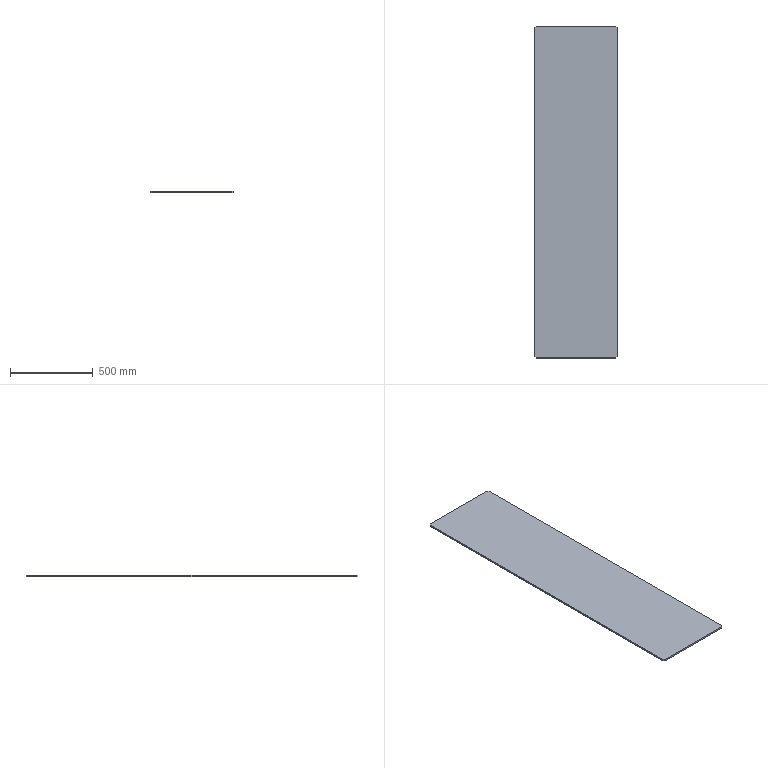Part | SolidWorks | features Chamfer 1, Extrusion 1 | 1 solid | 10 faces | box 500 x 2000 x 10 mm | volume 9998000 mm3 | plane 10
STEP:
#1=CARTESIAN_POINT('',(250.,-990.,5.));
#2=VERTEX_POINT('',#1);
#3=CARTESIAN_POINT('',(250.,990.,5.));
#4=VERTEX_POINT('',#3);
#5=CARTESIAN_POINT('',(250.,-1000.,5.));
#6=DIRECTION('',(0.,1.,0.));
#7=VECTOR('',#6,1000.);
#8=LINE('',#5,#7);
#9=EDGE_CURVE('',#2,#4,#8,.T.);
#10=ORIENTED_EDGE('',*,*,#9,.F.);
#11=CARTESIAN_POINT('',(250.,-990.,-5.));
#12=VERTEX_POINT('',#11);
#13=CARTESIAN_POINT('',(250.,-990.,5.));
#14=DIRECTION('',(0.,0.,-1.));
#15=VECTOR('',#14,1000.);
#16=LINE('',#13,#15);
#17=EDGE_CURVE('',#2,#12,#16,.T.);
#18=ORIENTED_EDGE('',*,*,#17,.T.);
#19=CARTESIAN_POINT('',(250.,990.,-5.));
#20=VERTEX_POINT('',#19);
#21=CARTESIAN_POINT('',(250.,-1000.,-5.));
#22=DIRECTION('',(0.,1.,0.));
#23=VECTOR('',#22,1000.);
#24=LINE('',#21,#23);
#25=EDGE_CURVE('',#12,#20,#24,.T.);
#26=ORIENTED_EDGE('',*,*,#25,.T.);
#27=CARTESIAN_POINT('',(250.,990.,5.));
#28=DIRECTION('',(0.,0.,1.));
#29=VECTOR('',#28,1000.);
#30=LINE('',#27,#29);
#31=EDGE_CURVE('',#20,#4,#30,.T.);
#32=ORIENTED_EDGE('',*,*,#31,.T.);
#33=EDGE_LOOP('',(#10,#18,#26,#32));
#34=FACE_OUTER_BOUND('',#33,.T.);
#35=CARTESIAN_POINT('',(250.,-1000.,5.));
#36=DIRECTION('',(-1.,0.,0.));
#37=DIRECTION('',(0.,0.,1.));
#38=AXIS2_PLACEMENT_3D('',#35,#36,#37);
#39=PLANE('',#38);
#40=ADVANCED_FACE('',(#34),#39,.F.);
#41=CARTESIAN_POINT('',(240.,1000.,-5.));
#42=VERTEX_POINT('',#41);
#43=CARTESIAN_POINT('',(-240.,1000.,-5.));
#44=VERTEX_POINT('',#43);
#45=CARTESIAN_POINT('',(-250.,1000.,-5.));
#46=DIRECTION('',(-1.,0.,0.));
#47=VECTOR('',#46,1000.);
#48=LINE('',#45,#47);
#49=EDGE_CURVE('',#42,#44,#48,.T.);
#50=ORIENTED_EDGE('',*,*,#49,.T.);
#51=CARTESIAN_POINT('',(-240.,1000.,5.));
#52=VERTEX_POINT('',#51);
#53=CARTESIAN_POINT('',(-240.,1000.,5.));
#54=DIRECTION('',(0.,0.,1.));
#55=VECTOR('',#54,1000.);
#56=LINE('',#53,#55);
#57=EDGE_CURVE('',#44,#52,#56,.T.);
#58=ORIENTED_EDGE('',*,*,#57,.T.);
#59=CARTESIAN_POINT('',(240.,1000.,5.));
#60=VERTEX_POINT('',#59);
#61=CARTESIAN_POINT('',(-250.,1000.,5.));
#62=DIRECTION('',(-1.,0.,0.));
#63=VECTOR('',#62,1000.);
#64=LINE('',#61,#63);
#65=EDGE_CURVE('',#60,#52,#64,.T.);
#66=ORIENTED_EDGE('',*,*,#65,.F.);
#67=CARTESIAN_POINT('',(240.,1000.,5.));
#68=DIRECTION('',(0.,0.,-1.));
#69=VECTOR('',#68,1000.);
#70=LINE('',#67,#69);
#71=EDGE_CURVE('',#60,#42,#70,.T.);
#72=ORIENTED_EDGE('',*,*,#71,.T.);
#73=EDGE_LOOP('',(#50,#58,#66,#72));
#74=FACE_OUTER_BOUND('',#73,.T.);
#75=CARTESIAN_POINT('',(-250.,1000.,5.));
#76=DIRECTION('',(0.,-1.,0.));
#77=DIRECTION('',(0.,0.,-1.));
#78=AXIS2_PLACEMENT_3D('',#75,#76,#77);
#79=PLANE('',#78);
#80=ADVANCED_FACE('',(#74),#79,.F.);
#81=CARTESIAN_POINT('',(-250.,990.,5.));
#82=VERTEX_POINT('',#81);
#83=CARTESIAN_POINT('',(-250.,-990.,5.));
#84=VERTEX_POINT('',#83);
#85=CARTESIAN_POINT('',(-250.,-1000.,5.));
#86=DIRECTION('',(0.,-1.,0.));
#87=VECTOR('',#86,1000.);
#88=LINE('',#85,#87);
#89=EDGE_CURVE('',#82,#84,#88,.T.);
#90=ORIENTED_EDGE('',*,*,#89,.F.);
#91=CARTESIAN_POINT('',(-250.,990.,-5.));
#92=VERTEX_POINT('',#91);
#93=CARTESIAN_POINT('',(-250.,990.,5.));
#94=DIRECTION('',(0.,0.,-1.));
#95=VECTOR('',#94,1000.);
#96=LINE('',#93,#95);
#97=EDGE_CURVE('',#82,#92,#96,.T.);
#98=ORIENTED_EDGE('',*,*,#97,.T.);
#99=CARTESIAN_POINT('',(-250.,-990.,-5.));
#100=VERTEX_POINT('',#99);
#101=CARTESIAN_POINT('',(-250.,-1000.,-5.));
#102=DIRECTION('',(0.,-1.,0.));
#103=VECTOR('',#102,1000.);
#104=LINE('',#101,#103);
#105=EDGE_CURVE('',#92,#100,#104,.T.);
#106=ORIENTED_EDGE('',*,*,#105,.T.);
#107=CARTESIAN_POINT('',(-250.,-990.,5.));
#108=DIRECTION('',(0.,0.,1.));
#109=VECTOR('',#108,1000.);
#110=LINE('',#107,#109);
#111=EDGE_CURVE('',#100,#84,#110,.T.);
#112=ORIENTED_EDGE('',*,*,#111,.T.);
#113=EDGE_LOOP('',(#90,#98,#106,#112));
#114=FACE_OUTER_BOUND('',#113,.T.);
#115=CARTESIAN_POINT('',(-250.,-1000.,5.));
#116=DIRECTION('',(1.,0.,0.));
#117=DIRECTION('',(0.,0.,-1.));
#118=AXIS2_PLACEMENT_3D('',#115,#116,#117);
#119=PLANE('',#118);
#120=ADVANCED_FACE('',(#114),#119,.F.);
#121=CARTESIAN_POINT('',(-240.,-1000.,5.));
#122=VERTEX_POINT('',#121);
#123=CARTESIAN_POINT('',(240.,-1000.,5.));
#124=VERTEX_POINT('',#123);
#125=CARTESIAN_POINT('',(-250.,-1000.,5.));
#126=DIRECTION('',(1.,0.,0.));
#127=VECTOR('',#126,1000.);
#128=LINE('',#125,#127);
#129=EDGE_CURVE('',#122,#124,#128,.T.);
#130=ORIENTED_EDGE('',*,*,#129,.F.);
#131=CARTESIAN_POINT('',(-240.,-1000.,-5.));
#132=VERTEX_POINT('',#131);
#133=CARTESIAN_POINT('',(-240.,-1000.,5.));
#134=DIRECTION('',(0.,0.,-1.));
#135=VECTOR('',#134,1000.);
#136=LINE('',#133,#135);
#137=EDGE_CURVE('',#122,#132,#136,.T.);
#138=ORIENTED_EDGE('',*,*,#137,.T.);
#139=CARTESIAN_POINT('',(240.,-1000.,-5.));
#140=VERTEX_POINT('',#139);
#141=CARTESIAN_POINT('',(-250.,-1000.,-5.));
#142=DIRECTION('',(1.,0.,0.));
#143=VECTOR('',#142,1000.);
#144=LINE('',#141,#143);
#145=EDGE_CURVE('',#132,#140,#144,.T.);
#146=ORIENTED_EDGE('',*,*,#145,.T.);
#147=CARTESIAN_POINT('',(240.,-1000.,5.));
#148=DIRECTION('',(0.,0.,1.));
#149=VECTOR('',#148,1000.);
#150=LINE('',#147,#149);
#151=EDGE_CURVE('',#140,#124,#150,.T.);
#152=ORIENTED_EDGE('',*,*,#151,.T.);
#153=EDGE_LOOP('',(#130,#138,#146,#152));
#154=FACE_OUTER_BOUND('',#153,.T.);
#155=CARTESIAN_POINT('',(-250.,-1000.,5.));
#156=DIRECTION('',(0.,1.,0.));
#157=DIRECTION('',(0.,0.,1.));
#158=AXIS2_PLACEMENT_3D('',#155,#156,#157);
#159=PLANE('',#158);
#160=ADVANCED_FACE('',(#154),#159,.F.);
#161=ORIENTED_EDGE('',*,*,#65,.T.);
#162=CARTESIAN_POINT('',(-250.,990.,5.));
#163=DIRECTION('',(-0.7071,-0.7071,0.));
#164=VECTOR('',#163,1000.);
#165=LINE('',#162,#164);
#166=EDGE_CURVE('',#52,#82,#165,.T.);
#167=ORIENTED_EDGE('',*,*,#166,.T.);
#168=ORIENTED_EDGE('',*,*,#89,.T.);
#169=CARTESIAN_POINT('',(-240.,-1000.,5.));
#170=DIRECTION('',(0.7071,-0.7071,0.));
#171=VECTOR('',#170,1000.);
#172=LINE('',#169,#171);
#173=EDGE_CURVE('',#84,#122,#172,.T.);
#174=ORIENTED_EDGE('',*,*,#173,.T.);
#175=ORIENTED_EDGE('',*,*,#129,.T.);
#176=CARTESIAN_POINT('',(250.,-990.,5.));
#177=DIRECTION('',(0.7071,0.7071,0.));
#178=VECTOR('',#177,1000.);
#179=LINE('',#176,#178);
#180=EDGE_CURVE('',#124,#2,#179,.T.);
#181=ORIENTED_EDGE('',*,*,#180,.T.);
#182=ORIENTED_EDGE('',*,*,#9,.T.);
#183=CARTESIAN_POINT('',(240.,1000.,5.));
#184=DIRECTION('',(-0.7071,0.7071,0.));
#185=VECTOR('',#184,1000.);
#186=LINE('',#183,#185);
#187=EDGE_CURVE('',#4,#60,#186,.T.);
#188=ORIENTED_EDGE('',*,*,#187,.T.);
#189=EDGE_LOOP('',(#161,#167,#168,#174,#175,#181,#182,#188));
#190=FACE_OUTER_BOUND('',#189,.T.);
#191=CARTESIAN_POINT('',(0.,0.,5.));
#192=DIRECTION('',(0.,0.,-1.));
#193=DIRECTION('',(-1.,0.,0.));
#194=AXIS2_PLACEMENT_3D('',#191,#192,#193);
#195=PLANE('',#194);
#196=ADVANCED_FACE('',(#190),#195,.F.);
#197=ORIENTED_EDGE('',*,*,#105,.F.);
#198=CARTESIAN_POINT('',(-620.,620.,-5.));
#199=DIRECTION('',(0.7071,0.7071,0.));
#200=VECTOR('',#199,1000.);
#201=LINE('',#198,#200);
#202=EDGE_CURVE('',#92,#44,#201,.T.);
#203=ORIENTED_EDGE('',*,*,#202,.T.);
#204=ORIENTED_EDGE('',*,*,#49,.F.);
#205=CARTESIAN_POINT('',(620.,620.,-5.));
#206=DIRECTION('',(0.7071,-0.7071,0.));
#207=VECTOR('',#206,1000.);
#208=LINE('',#205,#207);
#209=EDGE_CURVE('',#42,#20,#208,.T.);
#210=ORIENTED_EDGE('',*,*,#209,.T.);
#211=ORIENTED_EDGE('',*,*,#25,.F.);
#212=CARTESIAN_POINT('',(620.,-620.,-5.));
#213=DIRECTION('',(-0.7071,-0.7071,0.));
#214=VECTOR('',#213,1000.);
#215=LINE('',#212,#214);
#216=EDGE_CURVE('',#12,#140,#215,.T.);
#217=ORIENTED_EDGE('',*,*,#216,.T.);
#218=ORIENTED_EDGE('',*,*,#145,.F.);
#219=CARTESIAN_POINT('',(-620.,-620.,-5.));
#220=DIRECTION('',(-0.7071,0.7071,0.));
#221=VECTOR('',#220,1000.);
#222=LINE('',#219,#221);
#223=EDGE_CURVE('',#132,#100,#222,.T.);
#224=ORIENTED_EDGE('',*,*,#223,.T.);
#225=EDGE_LOOP('',(#197,#203,#204,#210,#211,#217,#218,#224));
#226=FACE_OUTER_BOUND('',#225,.T.);
#227=CARTESIAN_POINT('',(0.,0.,-5.));
#228=DIRECTION('',(0.,0.,-1.));
#229=DIRECTION('',(-1.,0.,0.));
#230=AXIS2_PLACEMENT_3D('',#227,#228,#229);
#231=PLANE('',#230);
#232=ADVANCED_FACE('',(#226),#231,.T.);
#233=ORIENTED_EDGE('',*,*,#166,.F.);
#234=ORIENTED_EDGE('',*,*,#57,.F.);
#235=ORIENTED_EDGE('',*,*,#202,.F.);
#236=ORIENTED_EDGE('',*,*,#97,.F.);
#237=EDGE_LOOP('',(#233,#234,#235,#236));
#238=FACE_OUTER_BOUND('',#237,.T.);
#239=CARTESIAN_POINT('',(-250.,990.,5.));
#240=DIRECTION('',(0.7071,-0.7071,0.));
#241=DIRECTION('',(0.,0.,-1.));
#242=AXIS2_PLACEMENT_3D('',#239,#240,#241);
#243=PLANE('',#242);
#244=ADVANCED_FACE('',(#238),#243,.F.);
#245=ORIENTED_EDGE('',*,*,#173,.F.);
#246=ORIENTED_EDGE('',*,*,#111,.F.);
#247=ORIENTED_EDGE('',*,*,#223,.F.);
#248=ORIENTED_EDGE('',*,*,#137,.F.);
#249=EDGE_LOOP('',(#245,#246,#247,#248));
#250=FACE_OUTER_BOUND('',#249,.T.);
#251=CARTESIAN_POINT('',(-240.,-1000.,5.));
#252=DIRECTION('',(0.7071,0.7071,0.));
#253=DIRECTION('',(0.,0.,-1.));
#254=AXIS2_PLACEMENT_3D('',#251,#252,#253);
#255=PLANE('',#254);
#256=ADVANCED_FACE('',(#250),#255,.F.);
#257=ORIENTED_EDGE('',*,*,#180,.F.);
#258=ORIENTED_EDGE('',*,*,#151,.F.);
#259=ORIENTED_EDGE('',*,*,#216,.F.);
#260=ORIENTED_EDGE('',*,*,#17,.F.);
#261=EDGE_LOOP('',(#257,#258,#259,#260));
#262=FACE_OUTER_BOUND('',#261,.T.);
#263=CARTESIAN_POINT('',(250.,-990.,5.));
#264=DIRECTION('',(-0.7071,0.7071,0.));
#265=DIRECTION('',(0.,0.,-1.));
#266=AXIS2_PLACEMENT_3D('',#263,#264,#265);
#267=PLANE('',#266);
#268=ADVANCED_FACE('',(#262),#267,.F.);
#269=ORIENTED_EDGE('',*,*,#187,.F.);
#270=ORIENTED_EDGE('',*,*,#31,.F.);
#271=ORIENTED_EDGE('',*,*,#209,.F.);
#272=ORIENTED_EDGE('',*,*,#71,.F.);
#273=EDGE_LOOP('',(#269,#270,#271,#272));
#274=FACE_OUTER_BOUND('',#273,.T.);
#275=CARTESIAN_POINT('',(240.,1000.,5.));
#276=DIRECTION('',(-0.7071,-0.7071,0.));
#277=DIRECTION('',(0.,0.,-1.));
#278=AXIS2_PLACEMENT_3D('',#275,#276,#277);
#279=PLANE('',#278);
#280=ADVANCED_FACE('',(#274),#279,.F.);
#281=CLOSED_SHELL('',(#40,#80,#120,#160,#196,#232,#244,#256,#268,#280));
#282=MANIFOLD_SOLID_BREP('',#281);
#283=CARTESIAN_POINT('',(0.,0.,0.));
#284=DIRECTION('',(0.,0.,1.));
#285=DIRECTION('',(1.,0.,0.));
#286=AXIS2_PLACEMENT_3D('',#283,#284,#285);
#287=(LENGTH_UNIT()NAMED_UNIT(*)SI_UNIT(.MILLI.,.METRE.));
#288=UNCERTAINTY_MEASURE_WITH_UNIT(LENGTH_MEASURE(0.00001),#287,'','');
#289=(NAMED_UNIT(*)PLANE_ANGLE_UNIT()SI_UNIT($,.RADIAN.));
#290=(NAMED_UNIT(*)SI_UNIT($,.STERADIAN.)SOLID_ANGLE_UNIT());
#291=(GEOMETRIC_REPRESENTATION_CONTEXT(3)GLOBAL_UNCERTAINTY_ASSIGNED_CONTEXT((#288))GLOBAL_UNIT_ASSIGNED_CONTEXT((#287,#289,#290))REPRESENTATION_CONTEXT('',''));
#292=ADVANCED_BREP_SHAPE_REPRESENTATION('',(#282,#286),#291);